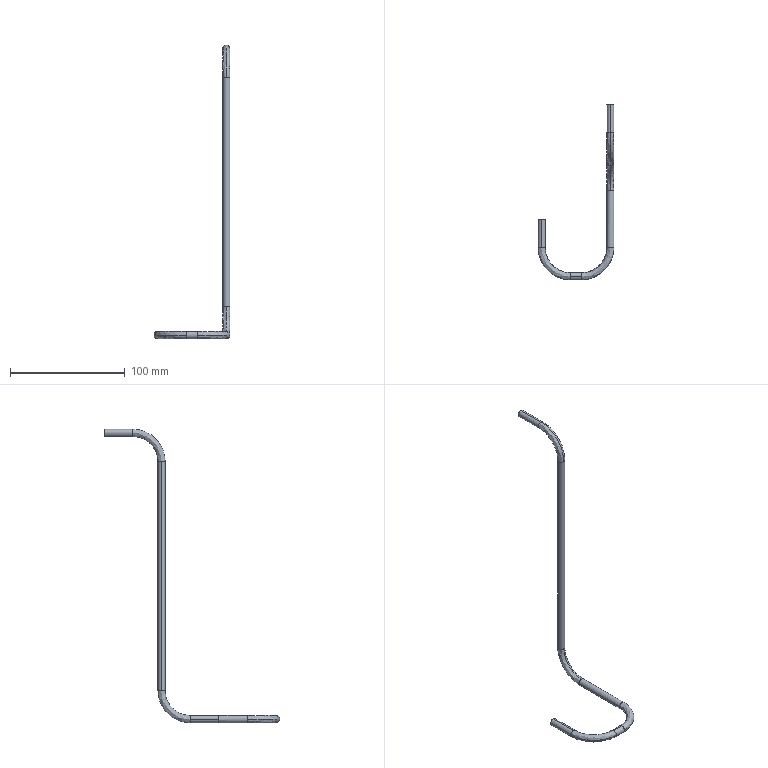Part | STEP file | copper tube 30_default_machined_ | 1 solid | 38 faces | box 66.35 x 153.175 x 256.35 mm | volume 6515 mm3 | cylinder 20 | spline 16 | plane 2 | commonest cylinder face diameters 4.75 x10 6.35 x10